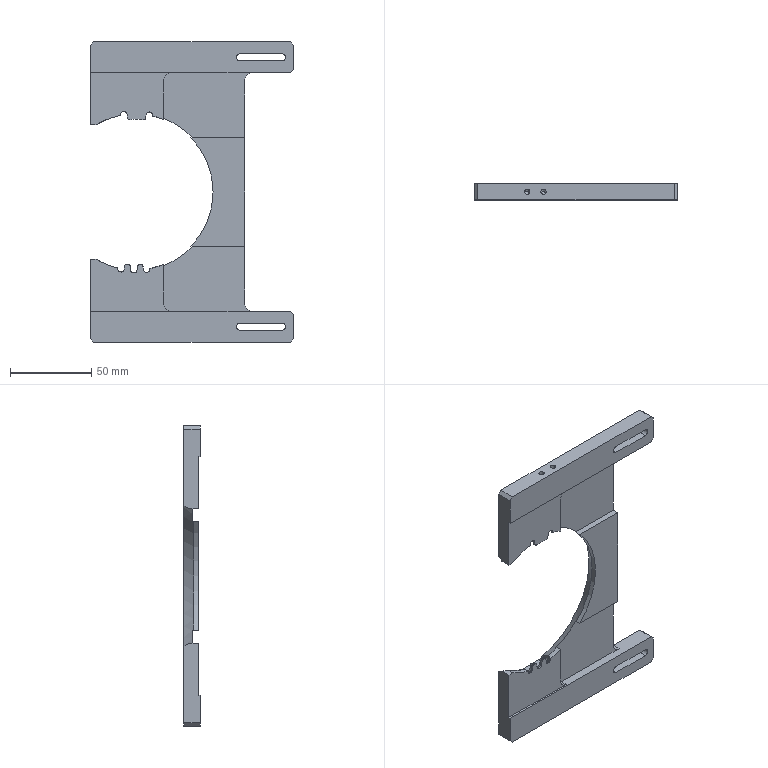Part | STEP file | material release guide plate | 1 solid | 138 faces | box 125 x 10 x 185 mm | volume 96002 mm3 | plane 59 | cylinder 49 | cone 30 | commonest cylinder face diameters 4 x10 3 x8 3.3 x8 96 x5 4.5 x4 8 x4